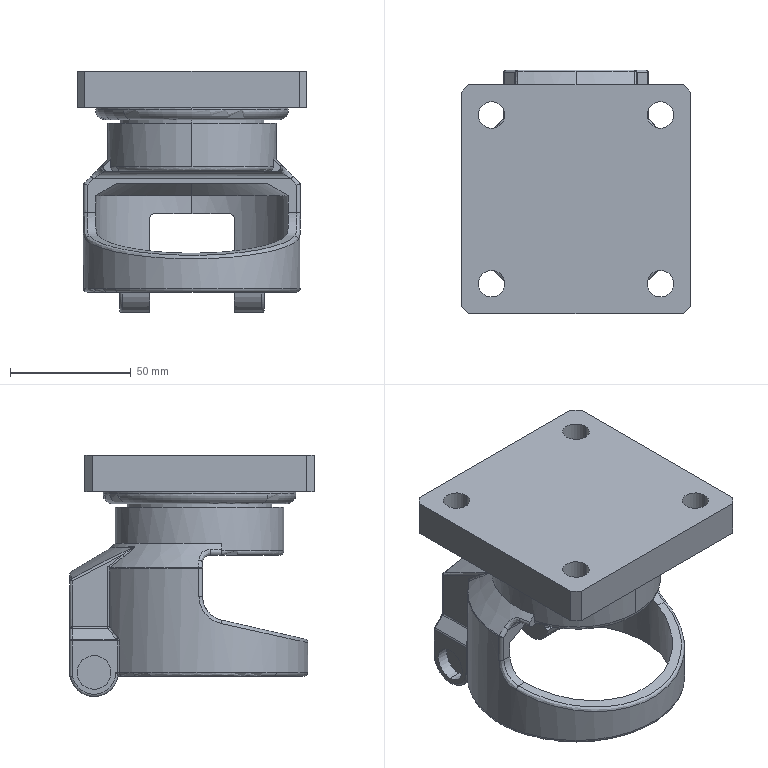Part | STEP file | ASND-0110-E63-HLTP01Clogo.sldasm-Part-215 | 1 solid | 144 faces | box 95 x 101.227 x 100 mm | volume 310497 mm3 | cylinder 54 | plane 35 | spline 25 | torus 18 | cone 6 | sphere 6 | commonest cylinder face diameters 2 x17 11 x8 3 x7 14 x4 20 x4 80 x4